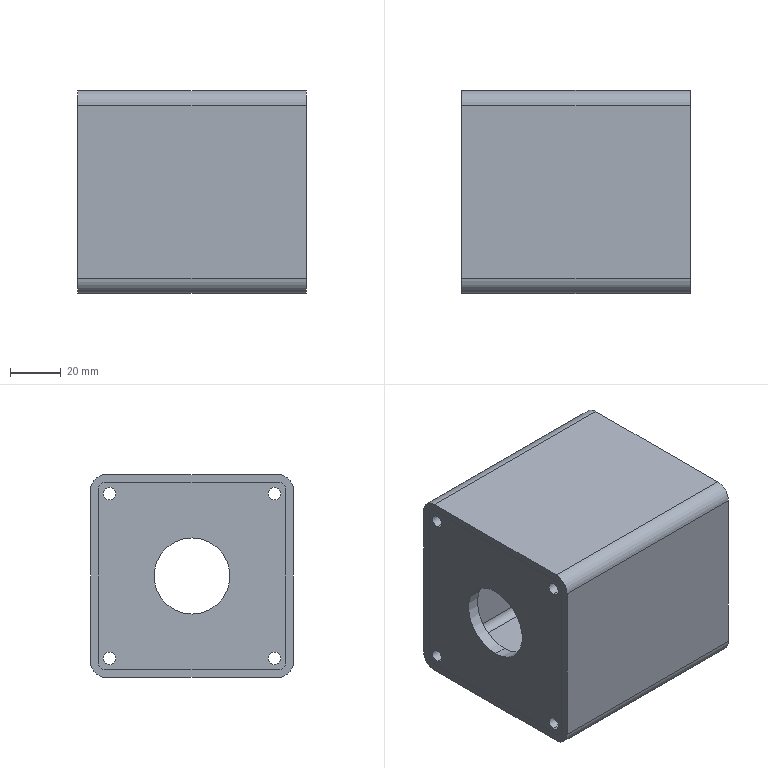Part | SolidWorks | features BaseBody 3 | 3 solids | 58 faces | box 90 x 80 x 80 mm | volume 127903 mm3 | cylinder 36 | plane 22 | commonest cylinder face diameters 5 x16 6 x12 12 x4 30 x4